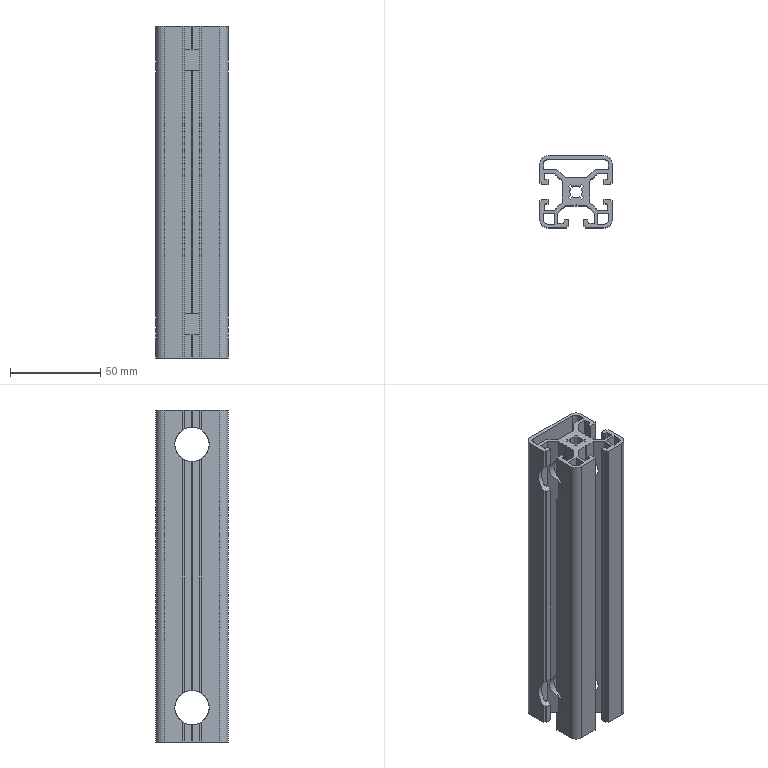Part | SolidWorks | features BaseBody 1, HoleWzd 1, MoveFace 1 | 1 solid | 242 faces | box 40 x 40 x 184 mm | volume 100557 mm3 | plane 187 | cylinder 55 | commonest cylinder face diameters 6.8 x15 2 x14 19 x12 1 x6 5 x4 9 x4